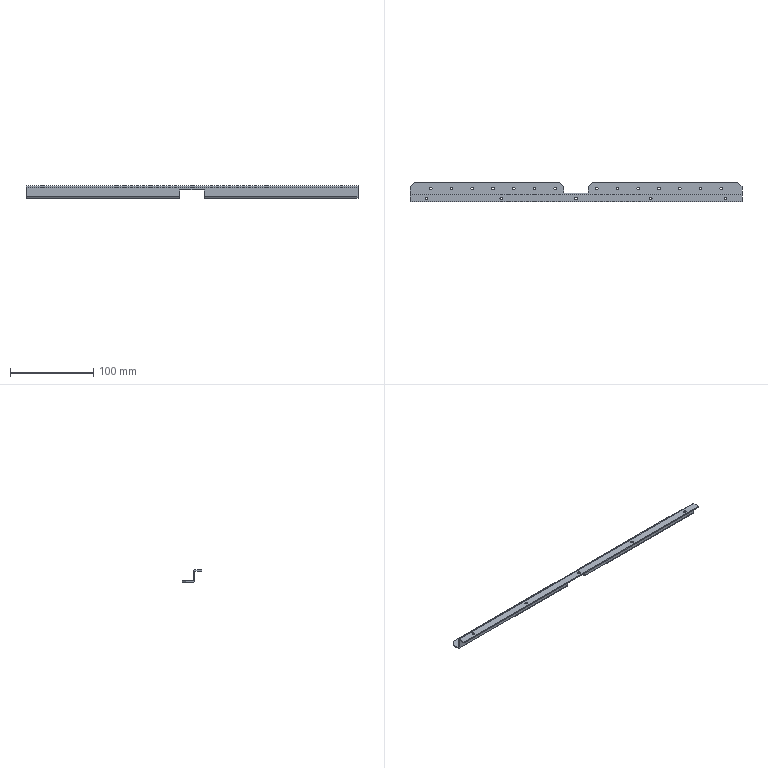Part | SolidWorks | features LPattern 4, ICE 3, EdgeFlange 2, Chamfer 1, FlatPattern 1, SMBaseFlange 1, SheetMetal 1 | 1 solid | 72 faces | box 400 x 23.5 x 15 mm | volume 20417 mm3 | cylinder 44 | plane 28 | commonest cylinder face diameters 3.2 x41 0.2 x3